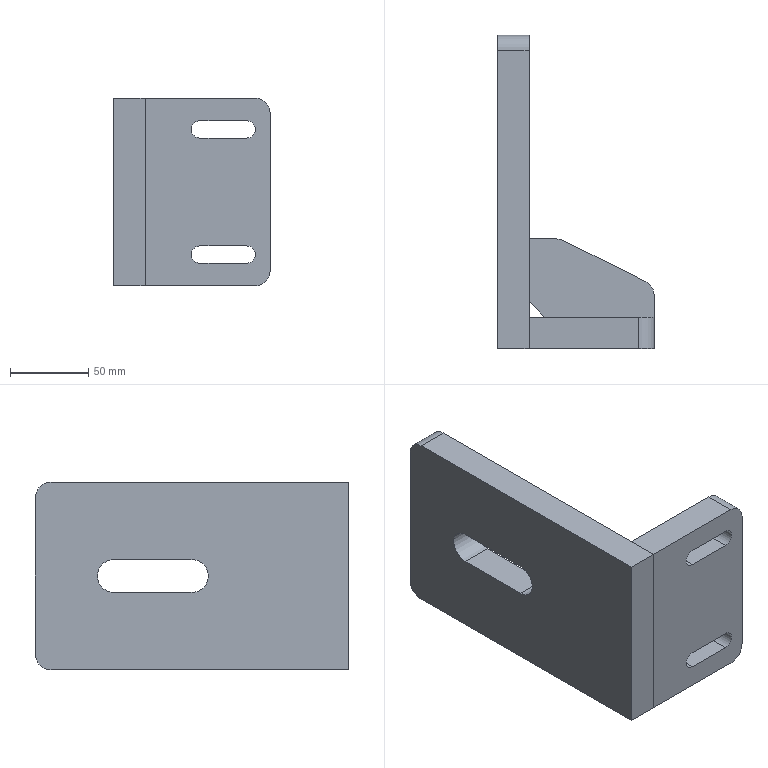Part | SolidWorks | features BaseBody 3 | 3 solids | 38 faces | box 100 x 200 x 120 mm | volume 655786 mm3 | plane 26 | cylinder 12 | commonest cylinder face diameters 20 x6 11 x4 21 x2
STEP:
#1=CARTESIAN_POINT('',(10.,-100.,-60.));
#2=VERTEX_POINT('',#1);
#3=CARTESIAN_POINT('',(10.,90.,-60.));
#4=VERTEX_POINT('',#3);
#5=CARTESIAN_POINT('',(10.,90.,-60.));
#6=DIRECTION('',(0.,1.,0.));
#7=VECTOR('',#6,1000.);
#8=LINE('',#5,#7);
#9=EDGE_CURVE('',#2,#4,#8,.T.);
#10=ORIENTED_EDGE('',*,*,#9,.T.);
#11=CARTESIAN_POINT('',(10.,100.,-50.));
#12=VERTEX_POINT('',#11);
#13=CARTESIAN_POINT('',(10.,90.,-50.));
#14=DIRECTION('',(1.,0.,0.));
#15=DIRECTION('',(0.,0.,1.));
#16=AXIS2_PLACEMENT_3D('',#13,#14,#15);
#17=CIRCLE('',#16,10.);
#18=EDGE_CURVE('',#4,#12,#17,.T.);
#19=ORIENTED_EDGE('',*,*,#18,.T.);
#20=CARTESIAN_POINT('',(10.,100.,50.));
#21=VERTEX_POINT('',#20);
#22=CARTESIAN_POINT('',(10.,100.,50.));
#23=DIRECTION('',(0.,0.,1.));
#24=VECTOR('',#23,1000.);
#25=LINE('',#22,#24);
#26=EDGE_CURVE('',#12,#21,#25,.T.);
#27=ORIENTED_EDGE('',*,*,#26,.T.);
#28=CARTESIAN_POINT('',(10.,90.,60.));
#29=VERTEX_POINT('',#28);
#30=CARTESIAN_POINT('',(10.,90.,50.));
#31=DIRECTION('',(1.,0.,0.));
#32=DIRECTION('',(0.,0.,-1.));
#33=AXIS2_PLACEMENT_3D('',#30,#31,#32);
#34=CIRCLE('',#33,10.);
#35=EDGE_CURVE('',#21,#29,#34,.T.);
#36=ORIENTED_EDGE('',*,*,#35,.T.);
#37=CARTESIAN_POINT('',(10.,-100.,60.));
#38=VERTEX_POINT('',#37);
#39=CARTESIAN_POINT('',(10.,90.,60.));
#40=DIRECTION('',(0.,-1.,0.));
#41=VECTOR('',#40,1000.);
#42=LINE('',#39,#41);
#43=EDGE_CURVE('',#29,#38,#42,.T.);
#44=ORIENTED_EDGE('',*,*,#43,.T.);
#45=CARTESIAN_POINT('',(10.,-100.,60.));
#46=DIRECTION('',(0.,0.,-1.));
#47=VECTOR('',#46,1000.);
#48=LINE('',#45,#47);
#49=EDGE_CURVE('',#38,#2,#48,.T.);
#50=ORIENTED_EDGE('',*,*,#49,.T.);
#51=EDGE_LOOP('',(#10,#19,#27,#36,#44,#50));
#52=FACE_OUTER_BOUND('',#51,.T.);
#53=CARTESIAN_POINT('',(10.,50.,10.5));
#54=VERTEX_POINT('',#53);
#55=CARTESIAN_POINT('',(10.,0.,10.5));
#56=VERTEX_POINT('',#55);
#57=CARTESIAN_POINT('',(10.,50.,10.5));
#58=DIRECTION('',(0.,-1.,0.));
#59=VECTOR('',#58,1000.);
#60=LINE('',#57,#59);
#61=EDGE_CURVE('',#54,#56,#60,.T.);
#62=ORIENTED_EDGE('',*,*,#61,.F.);
#63=CARTESIAN_POINT('',(10.,50.,-10.5));
#64=VERTEX_POINT('',#63);
#65=CARTESIAN_POINT('',(10.,50.,0.));
#66=DIRECTION('',(1.,0.,0.));
#67=DIRECTION('',(0.,0.,-1.));
#68=AXIS2_PLACEMENT_3D('',#65,#66,#67);
#69=CIRCLE('',#68,10.5);
#70=EDGE_CURVE('',#64,#54,#69,.T.);
#71=ORIENTED_EDGE('',*,*,#70,.F.);
#72=CARTESIAN_POINT('',(10.,0.,-10.5));
#73=VERTEX_POINT('',#72);
#74=CARTESIAN_POINT('',(10.,50.,-10.5));
#75=DIRECTION('',(0.,1.,0.));
#76=VECTOR('',#75,1000.);
#77=LINE('',#74,#76);
#78=EDGE_CURVE('',#73,#64,#77,.T.);
#79=ORIENTED_EDGE('',*,*,#78,.F.);
#80=CARTESIAN_POINT('',(10.,0.,0.));
#81=DIRECTION('',(1.,0.,0.));
#82=DIRECTION('',(0.,0.,-1.));
#83=AXIS2_PLACEMENT_3D('',#80,#81,#82);
#84=CIRCLE('',#83,10.5);
#85=EDGE_CURVE('',#56,#73,#84,.T.);
#86=ORIENTED_EDGE('',*,*,#85,.F.);
#87=EDGE_LOOP('',(#62,#71,#79,#86));
#88=FACE_BOUND('',#87,.T.);
#89=CARTESIAN_POINT('',(10.,90.,50.));
#90=DIRECTION('',(1.,0.,0.));
#91=DIRECTION('',(0.,0.,-1.));
#92=AXIS2_PLACEMENT_3D('',#89,#90,#91);
#93=PLANE('',#92);
#94=ADVANCED_FACE('',(#52,#88),#93,.T.);
#95=CARTESIAN_POINT('',(-10.,-100.,-60.));
#96=VERTEX_POINT('',#95);
#97=CARTESIAN_POINT('',(-10.,90.,-60.));
#98=VERTEX_POINT('',#97);
#99=CARTESIAN_POINT('',(-10.,90.,-60.));
#100=DIRECTION('',(0.,1.,0.));
#101=VECTOR('',#100,1000.);
#102=LINE('',#99,#101);
#103=EDGE_CURVE('',#96,#98,#102,.T.);
#104=ORIENTED_EDGE('',*,*,#103,.F.);
#105=CARTESIAN_POINT('',(-10.,-100.,60.));
#106=VERTEX_POINT('',#105);
#107=CARTESIAN_POINT('',(-10.,-100.,60.));
#108=DIRECTION('',(0.,0.,-1.));
#109=VECTOR('',#108,1000.);
#110=LINE('',#107,#109);
#111=EDGE_CURVE('',#106,#96,#110,.T.);
#112=ORIENTED_EDGE('',*,*,#111,.F.);
#113=CARTESIAN_POINT('',(-10.,90.,60.));
#114=VERTEX_POINT('',#113);
#115=CARTESIAN_POINT('',(-10.,90.,60.));
#116=DIRECTION('',(0.,-1.,0.));
#117=VECTOR('',#116,1000.);
#118=LINE('',#115,#117);
#119=EDGE_CURVE('',#114,#106,#118,.T.);
#120=ORIENTED_EDGE('',*,*,#119,.F.);
#121=CARTESIAN_POINT('',(-10.,100.,50.));
#122=VERTEX_POINT('',#121);
#123=CARTESIAN_POINT('',(-10.,90.,50.));
#124=DIRECTION('',(1.,0.,0.));
#125=DIRECTION('',(0.,0.,-1.));
#126=AXIS2_PLACEMENT_3D('',#123,#124,#125);
#127=CIRCLE('',#126,10.);
#128=EDGE_CURVE('',#122,#114,#127,.T.);
#129=ORIENTED_EDGE('',*,*,#128,.F.);
#130=CARTESIAN_POINT('',(-10.,100.,-50.));
#131=VERTEX_POINT('',#130);
#132=CARTESIAN_POINT('',(-10.,100.,50.));
#133=DIRECTION('',(0.,0.,1.));
#134=VECTOR('',#133,1000.);
#135=LINE('',#132,#134);
#136=EDGE_CURVE('',#131,#122,#135,.T.);
#137=ORIENTED_EDGE('',*,*,#136,.F.);
#138=CARTESIAN_POINT('',(-10.,90.,-50.));
#139=DIRECTION('',(1.,0.,0.));
#140=DIRECTION('',(0.,0.,1.));
#141=AXIS2_PLACEMENT_3D('',#138,#139,#140);
#142=CIRCLE('',#141,10.);
#143=EDGE_CURVE('',#98,#131,#142,.T.);
#144=ORIENTED_EDGE('',*,*,#143,.F.);
#145=EDGE_LOOP('',(#104,#112,#120,#129,#137,#144));
#146=FACE_OUTER_BOUND('',#145,.T.);
#147=CARTESIAN_POINT('',(-10.,50.,-10.5));
#148=VERTEX_POINT('',#147);
#149=CARTESIAN_POINT('',(-10.,50.,10.5));
#150=VERTEX_POINT('',#149);
#151=CARTESIAN_POINT('',(-10.,50.,0.));
#152=DIRECTION('',(1.,0.,0.));
#153=DIRECTION('',(0.,0.,-1.));
#154=AXIS2_PLACEMENT_3D('',#151,#152,#153);
#155=CIRCLE('',#154,10.5);
#156=EDGE_CURVE('',#148,#150,#155,.T.);
#157=ORIENTED_EDGE('',*,*,#156,.T.);
#158=CARTESIAN_POINT('',(-10.,0.,10.5));
#159=VERTEX_POINT('',#158);
#160=CARTESIAN_POINT('',(-10.,50.,10.5));
#161=DIRECTION('',(0.,-1.,0.));
#162=VECTOR('',#161,1000.);
#163=LINE('',#160,#162);
#164=EDGE_CURVE('',#150,#159,#163,.T.);
#165=ORIENTED_EDGE('',*,*,#164,.T.);
#166=CARTESIAN_POINT('',(-10.,0.,-10.5));
#167=VERTEX_POINT('',#166);
#168=CARTESIAN_POINT('',(-10.,0.,0.));
#169=DIRECTION('',(1.,0.,0.));
#170=DIRECTION('',(0.,0.,-1.));
#171=AXIS2_PLACEMENT_3D('',#168,#169,#170);
#172=CIRCLE('',#171,10.5);
#173=EDGE_CURVE('',#159,#167,#172,.T.);
#174=ORIENTED_EDGE('',*,*,#173,.T.);
#175=CARTESIAN_POINT('',(-10.,50.,-10.5));
#176=DIRECTION('',(0.,1.,0.));
#177=VECTOR('',#176,1000.);
#178=LINE('',#175,#177);
#179=EDGE_CURVE('',#167,#148,#178,.T.);
#180=ORIENTED_EDGE('',*,*,#179,.T.);
#181=EDGE_LOOP('',(#157,#165,#174,#180));
#182=FACE_BOUND('',#181,.T.);
#183=CARTESIAN_POINT('',(-10.,90.,50.));
#184=DIRECTION('',(1.,0.,0.));
#185=DIRECTION('',(0.,0.,-1.));
#186=AXIS2_PLACEMENT_3D('',#183,#184,#185);
#187=PLANE('',#186);
#188=ADVANCED_FACE('',(#146,#182),#187,.F.);
#189=ORIENTED_EDGE('',*,*,#103,.T.);
#190=CARTESIAN_POINT('',(10.,90.,-60.));
#191=DIRECTION('',(-1.,0.,0.));
#192=VECTOR('',#191,1000.);
#193=LINE('',#190,#192);
#194=EDGE_CURVE('',#4,#98,#193,.T.);
#195=ORIENTED_EDGE('',*,*,#194,.F.);
#196=ORIENTED_EDGE('',*,*,#9,.F.);
#197=CARTESIAN_POINT('',(10.,-100.,-60.));
#198=DIRECTION('',(-1.,0.,0.));
#199=VECTOR('',#198,1000.);
#200=LINE('',#197,#199);
#201=EDGE_CURVE('',#2,#96,#200,.T.);
#202=ORIENTED_EDGE('',*,*,#201,.T.);
#203=EDGE_LOOP('',(#189,#195,#196,#202));
#204=FACE_OUTER_BOUND('',#203,.T.);
#205=CARTESIAN_POINT('',(10.,90.,-60.));
#206=DIRECTION('',(0.,0.,1.));
#207=DIRECTION('',(0.,-1.,0.));
#208=AXIS2_PLACEMENT_3D('',#205,#206,#207);
#209=PLANE('',#208);
#210=ADVANCED_FACE('',(#204),#209,.F.);
#211=ORIENTED_EDGE('',*,*,#143,.T.);
#212=CARTESIAN_POINT('',(10.,100.,-50.));
#213=DIRECTION('',(-1.,0.,0.));
#214=VECTOR('',#213,1000.);
#215=LINE('',#212,#214);
#216=EDGE_CURVE('',#12,#131,#215,.T.);
#217=ORIENTED_EDGE('',*,*,#216,.F.);
#218=ORIENTED_EDGE('',*,*,#18,.F.);
#219=ORIENTED_EDGE('',*,*,#194,.T.);
#220=EDGE_LOOP('',(#211,#217,#218,#219));
#221=FACE_OUTER_BOUND('',#220,.T.);
#222=CARTESIAN_POINT('',(10.,90.,-50.));
#223=DIRECTION('',(-1.,0.,0.));
#224=DIRECTION('',(0.,0.,1.));
#225=AXIS2_PLACEMENT_3D('',#222,#223,#224);
#226=CYLINDRICAL_SURFACE('',#225,10.);
#227=ADVANCED_FACE('',(#221),#226,.T.);
#228=ORIENTED_EDGE('',*,*,#136,.T.);
#229=CARTESIAN_POINT('',(10.,100.,50.));
#230=DIRECTION('',(-1.,0.,0.));
#231=VECTOR('',#230,1000.);
#232=LINE('',#229,#231);
#233=EDGE_CURVE('',#21,#122,#232,.T.);
#234=ORIENTED_EDGE('',*,*,#233,.F.);
#235=ORIENTED_EDGE('',*,*,#26,.F.);
#236=ORIENTED_EDGE('',*,*,#216,.T.);
#237=EDGE_LOOP('',(#228,#234,#235,#236));
#238=FACE_OUTER_BOUND('',#237,.T.);
#239=CARTESIAN_POINT('',(10.,100.,50.));
#240=DIRECTION('',(0.,-1.,0.));
#241=DIRECTION('',(0.,0.,-1.));
#242=AXIS2_PLACEMENT_3D('',#239,#240,#241);
#243=PLANE('',#242);
#244=ADVANCED_FACE('',(#238),#243,.F.);
#245=ORIENTED_EDGE('',*,*,#128,.T.);
#246=CARTESIAN_POINT('',(10.,90.,60.));
#247=DIRECTION('',(-1.,0.,0.));
#248=VECTOR('',#247,1000.);
#249=LINE('',#246,#248);
#250=EDGE_CURVE('',#29,#114,#249,.T.);
#251=ORIENTED_EDGE('',*,*,#250,.F.);
#252=ORIENTED_EDGE('',*,*,#35,.F.);
#253=ORIENTED_EDGE('',*,*,#233,.T.);
#254=EDGE_LOOP('',(#245,#251,#252,#253));
#255=FACE_OUTER_BOUND('',#254,.T.);
#256=CARTESIAN_POINT('',(10.,90.,50.));
#257=DIRECTION('',(-1.,0.,0.));
#258=DIRECTION('',(0.,0.,1.));
#259=AXIS2_PLACEMENT_3D('',#256,#257,#258);
#260=CYLINDRICAL_SURFACE('',#259,10.);
#261=ADVANCED_FACE('',(#255),#260,.T.);
#262=ORIENTED_EDGE('',*,*,#119,.T.);
#263=CARTESIAN_POINT('',(10.,-100.,60.));
#264=DIRECTION('',(-1.,0.,0.));
#265=VECTOR('',#264,1000.);
#266=LINE('',#263,#265);
#267=EDGE_CURVE('',#38,#106,#266,.T.);
#268=ORIENTED_EDGE('',*,*,#267,.F.);
#269=ORIENTED_EDGE('',*,*,#43,.F.);
#270=ORIENTED_EDGE('',*,*,#250,.T.);
#271=EDGE_LOOP('',(#262,#268,#269,#270));
#272=FACE_OUTER_BOUND('',#271,.T.);
#273=CARTESIAN_POINT('',(10.,90.,60.));
#274=DIRECTION('',(0.,0.,-1.));
#275=DIRECTION('',(0.,1.,0.));
#276=AXIS2_PLACEMENT_3D('',#273,#274,#275);
#277=PLANE('',#276);
#278=ADVANCED_FACE('',(#272),#277,.F.);
#279=ORIENTED_EDGE('',*,*,#111,.T.);
#280=ORIENTED_EDGE('',*,*,#201,.F.);
#281=ORIENTED_EDGE('',*,*,#49,.F.);
#282=ORIENTED_EDGE('',*,*,#267,.T.);
#283=EDGE_LOOP('',(#279,#280,#281,#282));
#284=FACE_OUTER_BOUND('',#283,.T.);
#285=CARTESIAN_POINT('',(10.,-100.,60.));
#286=DIRECTION('',(0.,1.,0.));
#287=DIRECTION('',(0.,0.,1.));
#288=AXIS2_PLACEMENT_3D('',#285,#286,#287);
#289=PLANE('',#288);
#290=ADVANCED_FACE('',(#284),#289,.F.);
#291=ORIENTED_EDGE('',*,*,#156,.F.);
#292=CARTESIAN_POINT('',(10.,50.,-10.5));
#293=DIRECTION('',(-1.,0.,0.));
#294=VECTOR('',#293,1000.);
#295=LINE('',#292,#294);
#296=EDGE_CURVE('',#64,#148,#295,.T.);
#297=ORIENTED_EDGE('',*,*,#296,.F.);
#298=ORIENTED_EDGE('',*,*,#70,.T.);
#299=CARTESIAN_POINT('',(10.,50.,10.5));
#300=DIRECTION('',(-1.,0.,0.));
#301=VECTOR('',#300,1000.);
#302=LINE('',#299,#301);
#303=EDGE_CURVE('',#54,#150,#302,.T.);
#304=ORIENTED_EDGE('',*,*,#303,.T.);
#305=EDGE_LOOP('',(#291,#297,#298,#304));
#306=FACE_OUTER_BOUND('',#305,.T.);
#307=CARTESIAN_POINT('',(10.,50.,0.));
#308=DIRECTION('',(-1.,0.,0.));
#309=DIRECTION('',(0.,0.,1.));
#310=AXIS2_PLACEMENT_3D('',#307,#308,#309);
#311=CYLINDRICAL_SURFACE('',#310,10.5);
#312=ADVANCED_FACE('',(#306),#311,.F.);
#313=ORIENTED_EDGE('',*,*,#164,.F.);
#314=ORIENTED_EDGE('',*,*,#303,.F.);
#315=ORIENTED_EDGE('',*,*,#61,.T.);
#316=CARTESIAN_POINT('',(10.,0.,10.5));
#317=DIRECTION('',(-1.,0.,0.));
#318=VECTOR('',#317,1000.);
#319=LINE('',#316,#318);
#320=EDGE_CURVE('',#56,#159,#319,.T.);
#321=ORIENTED_EDGE('',*,*,#320,.T.);
#322=EDGE_LOOP('',(#313,#314,#315,#321));
#323=FACE_OUTER_BOUND('',#322,.T.);
#324=CARTESIAN_POINT('',(10.,50.,10.5));
#325=DIRECTION('',(0.,0.,-1.));
#326=DIRECTION('',(0.,1.,0.));
#327=AXIS2_PLACEMENT_3D('',#324,#325,#326);
#328=PLANE('',#327);
#329=ADVANCED_FACE('',(#323),#328,.T.);
#330=ORIENTED_EDGE('',*,*,#173,.F.);
#331=ORIENTED_EDGE('',*,*,#320,.F.);
#332=ORIENTED_EDGE('',*,*,#85,.T.);
#333=CARTESIAN_POINT('',(10.,0.,-10.5));
#334=DIRECTION('',(-1.,0.,0.));
#335=VECTOR('',#334,1000.);
#336=LINE('',#333,#335);
#337=EDGE_CURVE('',#73,#167,#336,.T.);
#338=ORIENTED_EDGE('',*,*,#337,.T.);
#339=EDGE_LOOP('',(#330,#331,#332,#338));
#340=FACE_OUTER_BOUND('',#339,.T.);
#341=CARTESIAN_POINT('',(10.,0.,0.));
#342=DIRECTION('',(-1.,0.,0.));
#343=DIRECTION('',(0.,0.,1.));
#344=AXIS2_PLACEMENT_3D('',#341,#342,#343);
#345=CYLINDRICAL_SURFACE('',#344,10.5);
#346=ADVANCED_FACE('',(#340),#345,.F.);
#347=ORIENTED_EDGE('',*,*,#179,.F.);
#348=ORIENTED_EDGE('',*,*,#337,.F.);
#349=ORIENTED_EDGE('',*,*,#78,.T.);
#350=ORIENTED_EDGE('',*,*,#296,.T.);
#351=EDGE_LOOP('',(#347,#348,#349,#350));
#352=FACE_OUTER_BOUND('',#351,.T.);
#353=CARTESIAN_POINT('',(10.,50.,-10.5));
#354=DIRECTION('',(0.,0.,1.));
#355=DIRECTION('',(0.,-1.,0.));
#356=AXIS2_PLACEMENT_3D('',#353,#354,#355);
#357=PLANE('',#356);
#358=ADVANCED_FACE('',(#352),#357,.T.);
#359=CLOSED_SHELL('',(#94,#188,#210,#227,#244,#261,#278,#290,#312,#329,#346,#358));
#360=MANIFOLD_SOLID_BREP('',#359);
#361=CARTESIAN_POINT('',(80.,-100.,60.));
#362=VERTEX_POINT('',#361);
#363=CARTESIAN_POINT('',(10.,-100.,60.));
#364=VERTEX_POINT('',#363);
#365=CARTESIAN_POINT('',(90.,-100.,60.));
#366=DIRECTION('',(-1.,0.,0.));
#367=VECTOR('',#366,1000.);
#368=LINE('',#365,#367);
#369=EDGE_CURVE('',#362,#364,#368,.T.);
#370=ORIENTED_EDGE('',*,*,#369,.F.);
#371=CARTESIAN_POINT('',(80.,-80.,60.));
#372=VERTEX_POINT('',#371);
#373=CARTESIAN_POINT('',(80.,-100.,60.));
#374=DIRECTION('',(0.,1.,0.));
#375=VECTOR('',#374,1000.);
#376=LINE('',#373,#375);
#377=EDGE_CURVE('',#362,#372,#376,.T.);
#378=ORIENTED_EDGE('',*,*,#377,.T.);
#379=CARTESIAN_POINT('',(10.,-80.,60.));
#380=VERTEX_POINT('',#379);
#381=CARTESIAN_POINT('',(90.,-80.,60.));
#382=DIRECTION('',(-1.,0.,0.));
#383=VECTOR('',#382,1000.);
#384=LINE('',#381,#383);
#385=EDGE_CURVE('',#372,#380,#384,.T.);
#386=ORIENTED_EDGE('',*,*,#385,.T.);
#387=CARTESIAN_POINT('',(10.,-100.,60.));
#388=DIRECTION('',(0.,-1.,0.));
#389=VECTOR('',#388,1000.);
#390=LINE('',#387,#389);
#391=EDGE_CURVE('',#380,#364,#390,.T.);
#392=ORIENTED_EDGE('',*,*,#391,.T.);
#393=EDGE_LOOP('',(#370,#378,#386,#392));
#394=FACE_OUTER_BOUND('',#393,.T.);
#395=CARTESIAN_POINT('',(90.,-100.,60.));
#396=DIRECTION('',(0.,0.,-1.));
#397=DIRECTION('',(-1.,0.,0.));
#398=AXIS2_PLACEMENT_3D('',#395,#396,#397);
#399=PLANE('',#398);
#400=ADVANCED_FACE('',(#394),#399,.F.);
#401=CARTESIAN_POINT('',(75.,-100.,-45.5));
#402=VERTEX_POINT('',#401);
#403=CARTESIAN_POINT('',(45.,-100.,-45.5));
#404=VERTEX_POINT('',#403);
#405=CARTESIAN_POINT('',(90.,-100.,-45.5));
#406=DIRECTION('',(-1.,0.,0.));
#407=VECTOR('',#406,1000.);
#408=LINE('',#405,#407);
#409=EDGE_CURVE('',#402,#404,#408,.T.);
#410=ORIENTED_EDGE('',*,*,#409,.T.);
#411=CARTESIAN_POINT('',(45.,-100.,-34.5));
#412=VERTEX_POINT('',#411);
#413=CARTESIAN_POINT('',(45.,-100.,-40.));
#414=DIRECTION('',(0.,1.,0.));
#415=DIRECTION('',(0.,0.,1.));
#416=AXIS2_PLACEMENT_3D('',#413,#414,#415);
#417=CIRCLE('',#416,5.5);
#418=EDGE_CURVE('',#404,#412,#417,.T.);
#419=ORIENTED_EDGE('',*,*,#418,.T.);
#420=CARTESIAN_POINT('',(75.,-100.,-34.5));
#421=VERTEX_POINT('',#420);
#422=CARTESIAN_POINT('',(90.,-100.,-34.5));
#423=DIRECTION('',(1.,0.,0.));
#424=VECTOR('',#423,1000.);
#425=LINE('',#422,#424);
#426=EDGE_CURVE('',#412,#421,#425,.T.);
#427=ORIENTED_EDGE('',*,*,#426,.T.);
#428=CARTESIAN_POINT('',(75.,-100.,-40.));
#429=DIRECTION('',(0.,1.,0.));
#430=DIRECTION('',(0.,0.,1.));
#431=AXIS2_PLACEMENT_3D('',#428,#429,#430);
#432=CIRCLE('',#431,5.5);
#433=EDGE_CURVE('',#421,#402,#432,.T.);
#434=ORIENTED_EDGE('',*,*,#433,.T.);
#435=EDGE_LOOP('',(#410,#419,#427,#434));
#436=FACE_BOUND('',#435,.T.);
#437=CARTESIAN_POINT('',(75.,-100.,34.5));
#438=VERTEX_POINT('',#437);
#439=CARTESIAN_POINT('',(45.,-100.,34.5));
#440=VERTEX_POINT('',#439);
#441=CARTESIAN_POINT('',(90.,-100.,34.5));
#442=DIRECTION('',(-1.,0.,0.));
#443=VECTOR('',#442,1000.);
#444=LINE('',#441,#443);
#445=EDGE_CURVE('',#438,#440,#444,.T.);
#446=ORIENTED_EDGE('',*,*,#445,.T.);
#447=CARTESIAN_POINT('',(45.,-100.,45.5));
#448=VERTEX_POINT('',#447);
#449=CARTESIAN_POINT('',(45.,-100.,40.));
#450=DIRECTION('',(0.,1.,0.));
#451=DIRECTION('',(0.,0.,1.));
#452=AXIS2_PLACEMENT_3D('',#449,#450,#451);
#453=CIRCLE('',#452,5.5);
#454=EDGE_CURVE('',#440,#448,#453,.T.);
#455=ORIENTED_EDGE('',*,*,#454,.T.);
#456=CARTESIAN_POINT('',(75.,-100.,45.5));
#457=VERTEX_POINT('',#456);
#458=CARTESIAN_POINT('',(90.,-100.,45.5));
#459=DIRECTION('',(1.,0.,0.));
#460=VECTOR('',#459,1000.);
#461=LINE('',#458,#460);
#462=EDGE_CURVE('',#448,#457,#461,.T.);
#463=ORIENTED_EDGE('',*,*,#462,.T.);
#464=CARTESIAN_POINT('',(75.,-100.,40.));
#465=DIRECTION('',(0.,1.,0.));
#466=DIRECTION('',(0.,0.,1.));
#467=AXIS2_PLACEMENT_3D('',#464,#465,#466);
#468=CIRCLE('',#467,5.5);
#469=EDGE_CURVE('',#457,#438,#468,.T.);
#470=ORIENTED_EDGE('',*,*,#469,.T.);
#471=EDGE_LOOP('',(#446,#455,#463,#470));
#472=FACE_BOUND('',#471,.T.);
#473=CARTESIAN_POINT('',(90.,-100.,50.));
#474=VERTEX_POINT('',#473);
#475=CARTESIAN_POINT('',(90.,-100.,-50.));
#476=VERTEX_POINT('',#475);
#477=CARTESIAN_POINT('',(90.,-100.,60.));
#478=DIRECTION('',(0.,0.,-1.));
#479=VECTOR('',#478,1000.);
#480=LINE('',#477,#479);
#481=EDGE_CURVE('',#474,#476,#480,.T.);
#482=ORIENTED_EDGE('',*,*,#481,.F.);
#483=CARTESIAN_POINT('',(80.,-100.,50.));
#484=DIRECTION('',(0.,-1.,0.));
#485=DIRECTION('',(0.,0.,1.));
#486=AXIS2_PLACEMENT_3D('',#483,#484,#485);
#487=CIRCLE('',#486,10.);
#488=EDGE_CURVE('',#474,#362,#487,.T.);
#489=ORIENTED_EDGE('',*,*,#488,.T.);
#490=ORIENTED_EDGE('',*,*,#369,.T.);
#491=CARTESIAN_POINT('',(10.,-100.,-60.));
#492=VERTEX_POINT('',#491);
#493=CARTESIAN_POINT('',(10.,-100.,60.));
#494=DIRECTION('',(0.,0.,-1.));
#495=VECTOR('',#494,1000.);
#496=LINE('',#493,#495);
#497=EDGE_CURVE('',#364,#492,#496,.T.);
#498=ORIENTED_EDGE('',*,*,#497,.T.);
#499=CARTESIAN_POINT('',(80.,-100.,-60.));
#500=VERTEX_POINT('',#499);
#501=CARTESIAN_POINT('',(90.,-100.,-60.));
#502=DIRECTION('',(-1.,0.,0.));
#503=VECTOR('',#502,1000.);
#504=LINE('',#501,#503);
#505=EDGE_CURVE('',#500,#492,#504,.T.);
#506=ORIENTED_EDGE('',*,*,#505,.F.);
#507=CARTESIAN_POINT('',(80.,-100.,-50.));
#508=DIRECTION('',(0.,-1.,0.));
#509=DIRECTION('',(0.,0.,1.));
#510=AXIS2_PLACEMENT_3D('',#507,#508,#509);
#511=CIRCLE('',#510,10.);
#512=EDGE_CURVE('',#500,#476,#511,.T.);
#513=ORIENTED_EDGE('',*,*,#512,.T.);
#514=EDGE_LOOP('',(#482,#489,#490,#498,#506,#513));
#515=FACE_OUTER_BOUND('',#514,.T.);
#516=CARTESIAN_POINT('',(90.,-100.,60.));
#517=DIRECTION('',(0.,1.,0.));
#518=DIRECTION('',(0.,0.,1.));
#519=AXIS2_PLACEMENT_3D('',#516,#517,#518);
#520=PLANE('',#519);
#521=ADVANCED_FACE('',(#436,#472,#515),#520,.F.);
#522=CARTESIAN_POINT('',(80.,-80.,-60.));
#523=VERTEX_POINT('',#522);
#524=CARTESIAN_POINT('',(10.,-80.,-60.));
#525=VERTEX_POINT('',#524);
#526=CARTESIAN_POINT('',(90.,-80.,-60.));
#527=DIRECTION('',(-1.,0.,0.));
#528=VECTOR('',#527,1000.);
#529=LINE('',#526,#528);
#530=EDGE_CURVE('',#523,#525,#529,.T.);
#531=ORIENTED_EDGE('',*,*,#530,.F.);
#532=CARTESIAN_POINT('',(80.,-100.,-60.));
#533=DIRECTION('',(0.,-1.,0.));
#534=VECTOR('',#533,1000.);
#535=LINE('',#532,#534);
#536=EDGE_CURVE('',#523,#500,#535,.T.);
#537=ORIENTED_EDGE('',*,*,#536,.T.);
#538=ORIENTED_EDGE('',*,*,#505,.T.);
#539=CARTESIAN_POINT('',(10.,-100.,-60.));
#540=DIRECTION('',(0.,1.,0.));
#541=VECTOR('',#540,1000.);
#542=LINE('',#539,#541);
#543=EDGE_CURVE('',#492,#525,#542,.T.);
#544=ORIENTED_EDGE('',*,*,#543,.T.);
#545=EDGE_LOOP('',(#531,#537,#538,#544));
#546=FACE_OUTER_BOUND('',#545,.T.);
#547=CARTESIAN_POINT('',(90.,-100.,-60.));
#548=DIRECTION('',(0.,0.,1.));
#549=DIRECTION('',(0.,-1.,0.));
#550=AXIS2_PLACEMENT_3D('',#547,#548,#549);
#551=PLANE('',#550);
#552=ADVANCED_FACE('',(#546),#551,.F.);
#553=CARTESIAN_POINT('',(45.,-80.,-34.5));
#554=VERTEX_POINT('',#553);
#555=CARTESIAN_POINT('',(75.,-80.,-34.5));
#556=VERTEX_POINT('',#555);
#557=CARTESIAN_POINT('',(45.,-80.,-34.5));
#558=DIRECTION('',(1.,0.,0.));
#559=VECTOR('',#558,1000.);
#560=LINE('',#557,#559);
#561=EDGE_CURVE('',#554,#556,#560,.T.);
#562=ORIENTED_EDGE('',*,*,#561,.F.);
#563=CARTESIAN_POINT('',(45.,-80.,-45.5));
#564=VERTEX_POINT('',#563);
#565=CARTESIAN_POINT('',(45.,-80.,-40.));
#566=DIRECTION('',(0.,1.,0.));
#567=DIRECTION('',(0.,0.,1.));
#568=AXIS2_PLACEMENT_3D('',#565,#566,#567);
#569=CIRCLE('',#568,5.5);
#570=EDGE_CURVE('',#564,#554,#569,.T.);
#571=ORIENTED_EDGE('',*,*,#570,.F.);
#572=CARTESIAN_POINT('',(75.,-80.,-45.5));
#573=VERTEX_POINT('',#572);
#574=CARTESIAN_POINT('',(45.,-80.,-45.5));
#575=DIRECTION('',(-1.,0.,0.));
#576=VECTOR('',#575,1000.);
#577=LINE('',#574,#576);
#578=EDGE_CURVE('',#573,#564,#577,.T.);
#579=ORIENTED_EDGE('',*,*,#578,.F.);
#580=CARTESIAN_POINT('',(75.,-80.,-40.));
#581=DIRECTION('',(0.,1.,0.));
#582=DIRECTION('',(0.,0.,1.));
#583=AXIS2_PLACEMENT_3D('',#580,#581,#582);
#584=CIRCLE('',#583,5.5);
#585=EDGE_CURVE('',#556,#573,#584,.T.);
#586=ORIENTED_EDGE('',*,*,#585,.F.);
#587=EDGE_LOOP('',(#562,#571,#579,#586));
#588=FACE_BOUND('',#587,.T.);
#589=CARTESIAN_POINT('',(45.,-80.,45.5));
#590=VERTEX_POINT('',#589);
#591=CARTESIAN_POINT('',(75.,-80.,45.5));
#592=VERTEX_POINT('',#591);
#593=CARTESIAN_POINT('',(45.,-80.,45.5));
#594=DIRECTION('',(1.,0.,0.));
#595=VECTOR('',#594,1000.);
#596=LINE('',#593,#595);
#597=EDGE_CURVE('',#590,#592,#596,.T.);
#598=ORIENTED_EDGE('',*,*,#597,.F.);
#599=CARTESIAN_POINT('',(45.,-80.,34.5));
#600=VERTEX_POINT('',#599);
#601=CARTESIAN_POINT('',(45.,-80.,40.));
#602=DIRECTION('',(0.,1.,0.));
#603=DIRECTION('',(0.,0.,1.));
#604=AXIS2_PLACEMENT_3D('',#601,#602,#603);
#605=CIRCLE('',#604,5.5);
#606=EDGE_CURVE('',#600,#590,#605,.T.);
#607=ORIENTED_EDGE('',*,*,#606,.F.);
#608=CARTESIAN_POINT('',(75.,-80.,34.5));
#609=VERTEX_POINT('',#608);
#610=CARTESIAN_POINT('',(45.,-80.,34.5));
#611=DIRECTION('',(-1.,0.,0.));
#612=VECTOR('',#611,1000.);
#613=LINE('',#610,#612);
#614=EDGE_CURVE('',#609,#600,#613,.T.);
#615=ORIENTED_EDGE('',*,*,#614,.F.);
#616=CARTESIAN_POINT('',(75.,-80.,40.));
#617=DIRECTION('',(0.,1.,0.));
#618=DIRECTION('',(0.,0.,1.));
#619=AXIS2_PLACEMENT_3D('',#616,#617,#618);
#620=CIRCLE('',#619,5.5);
#621=EDGE_CURVE('',#592,#609,#620,.T.);
#622=ORIENTED_EDGE('',*,*,#621,.F.);
#623=EDGE_LOOP('',(#598,#607,#615,#622));
#624=FACE_BOUND('',#623,.T.);
#625=ORIENTED_EDGE('',*,*,#385,.F.);
#626=CARTESIAN_POINT('',(90.,-80.,50.));
#627=VERTEX_POINT('',#626);
#628=CARTESIAN_POINT('',(80.,-80.,50.));
#629=DIRECTION('',(0.,1.,0.));
#630=DIRECTION('',(0.,0.,-1.));
#631=AXIS2_PLACEMENT_3D('',#628,#629,#630);
#632=CIRCLE('',#631,10.);
#633=EDGE_CURVE('',#372,#627,#632,.T.);
#634=ORIENTED_EDGE('',*,*,#633,.T.);
#635=CARTESIAN_POINT('',(90.,-80.,-50.));
#636=VERTEX_POINT('',#635);
#637=CARTESIAN_POINT('',(90.,-80.,60.));
#638=DIRECTION('',(0.,0.,1.));
#639=VECTOR('',#638,1000.);
#640=LINE('',#637,#639);
#641=EDGE_CURVE('',#636,#627,#640,.T.);
#642=ORIENTED_EDGE('',*,*,#641,.F.);
#643=CARTESIAN_POINT('',(80.,-80.,-50.));
#644=DIRECTION('',(0.,1.,0.));
#645=DIRECTION('',(0.,0.,-1.));
#646=AXIS2_PLACEMENT_3D('',#643,#644,#645);
#647=CIRCLE('',#646,10.);
#648=EDGE_CURVE('',#636,#523,#647,.T.);
#649=ORIENTED_EDGE('',*,*,#648,.T.);
#650=ORIENTED_EDGE('',*,*,#530,.T.);
#651=CARTESIAN_POINT('',(10.,-80.,60.));
#652=DIRECTION('',(0.,0.,1.));
#653=VECTOR('',#652,1000.);
#654=LINE('',#651,#653);
#655=EDGE_CURVE('',#525,#380,#654,.T.);
#656=ORIENTED_EDGE('',*,*,#655,.T.);
#657=EDGE_LOOP('',(#625,#634,#642,#649,#650,#656));
#658=FACE_OUTER_BOUND('',#657,.T.);
#659=CARTESIAN_POINT('',(90.,-80.,60.));
#660=DIRECTION('',(0.,-1.,0.));
#661=DIRECTION('',(0.,0.,-1.));
#662=AXIS2_PLACEMENT_3D('',#659,#660,#661);
#663=PLANE('',#662);
#664=ADVANCED_FACE('',(#588,#624,#658),#663,.F.);
#665=ORIENTED_EDGE('',*,*,#641,.T.);
#666=CARTESIAN_POINT('',(90.,0.,50.));
#667=DIRECTION('',(0.,-1.,0.));
#668=VECTOR('',#667,1000.);
#669=LINE('',#666,#668);
#670=EDGE_CURVE('',#627,#474,#669,.T.);
#671=ORIENTED_EDGE('',*,*,#670,.T.);
#672=ORIENTED_EDGE('',*,*,#481,.T.);
#673=CARTESIAN_POINT('',(90.,0.,-50.));
#674=DIRECTION('',(0.,1.,0.));
#675=VECTOR('',#674,1000.);
#676=LINE('',#673,#675);
#677=EDGE_CURVE('',#476,#636,#676,.T.);
#678=ORIENTED_EDGE('',*,*,#677,.T.);
#679=EDGE_LOOP('',(#665,#671,#672,#678));
#680=FACE_OUTER_BOUND('',#679,.T.);
#681=CARTESIAN_POINT('',(90.,0.,0.));
#682=DIRECTION('',(-1.,0.,0.));
#683=DIRECTION('',(0.,0.,1.));
#684=AXIS2_PLACEMENT_3D('',#681,#682,#683);
#685=PLANE('',#684);
#686=ADVANCED_FACE('',(#680),#685,.F.);
#687=ORIENTED_EDGE('',*,*,#391,.F.);
#688=ORIENTED_EDGE('',*,*,#655,.F.);
#689=ORIENTED_EDGE('',*,*,#543,.F.);
#690=ORIENTED_EDGE('',*,*,#497,.F.);
#691=EDGE_LOOP('',(#687,#688,#689,#690));
#692=FACE_OUTER_BOUND('',#691,.T.);
#693=CARTESIAN_POINT('',(10.,0.,0.));
#694=DIRECTION('',(-1.,0.,0.));
#695=DIRECTION('',(0.,0.,1.));
#696=AXIS2_PLACEMENT_3D('',#693,#694,#695);
#697=PLANE('',#696);
#698=ADVANCED_FACE('',(#692),#697,.T.);
#699=ORIENTED_EDGE('',*,*,#633,.F.);
#700=ORIENTED_EDGE('',*,*,#377,.F.);
#701=ORIENTED_EDGE('',*,*,#488,.F.);
#702=ORIENTED_EDGE('',*,*,#670,.F.);
#703=EDGE_LOOP('',(#699,#700,#701,#702));
#704=FACE_OUTER_BOUND('',#703,.T.);
#705=CARTESIAN_POINT('',(80.,0.,50.));
#706=DIRECTION('',(0.,-1.,0.));
#707=DIRECTION('',(0.,0.,-1.));
#708=AXIS2_PLACEMENT_3D('',#705,#706,#707);
#709=CYLINDRICAL_SURFACE('',#708,10.);
#710=ADVANCED_FACE('',(#704),#709,.T.);
#711=ORIENTED_EDGE('',*,*,#512,.F.);
#712=ORIENTED_EDGE('',*,*,#536,.F.);
#713=ORIENTED_EDGE('',*,*,#648,.F.);
#714=ORIENTED_EDGE('',*,*,#677,.F.);
#715=EDGE_LOOP('',(#711,#712,#713,#714));
#716=FACE_OUTER_BOUND('',#715,.T.);
#717=CARTESIAN_POINT('',(80.,0.,-50.));
#718=DIRECTION('',(0.,1.,0.));
#719=DIRECTION('',(0.,0.,1.));
#720=AXIS2_PLACEMENT_3D('',#717,#718,#719);
#721=CYLINDRICAL_SURFACE('',#720,10.);
#722=ADVANCED_FACE('',(#716),#721,.T.);
#723=CARTESIAN_POINT('',(45.,-140.,34.5));
#724=DIRECTION('',(0.,1.,0.));
#725=VECTOR('',#724,1000.);
#726=LINE('',#723,#725);
#727=EDGE_CURVE('',#440,#600,#726,.T.);
#728=ORIENTED_EDGE('',*,*,#727,.T.);
#729=ORIENTED_EDGE('',*,*,#606,.T.);
#730=CARTESIAN_POINT('',(45.,-140.,45.5));
#731=DIRECTION('',(0.,1.,0.));
#732=VECTOR('',#731,1000.);
#733=LINE('',#730,#732);
#734=EDGE_CURVE('',#448,#590,#733,.T.);
#735=ORIENTED_EDGE('',*,*,#734,.F.);
#736=ORIENTED_EDGE('',*,*,#454,.F.);
#737=EDGE_LOOP('',(#728,#729,#735,#736));
#738=FACE_OUTER_BOUND('',#737,.T.);
#739=CARTESIAN_POINT('',(45.,-140.,40.));
#740=DIRECTION('',(0.,1.,0.));
#741=DIRECTION('',(0.,0.,1.));
#742=AXIS2_PLACEMENT_3D('',#739,#740,#741);
#743=CYLINDRICAL_SURFACE('',#742,5.5);
#744=ADVANCED_FACE('',(#738),#743,.F.);
#745=CARTESIAN_POINT('',(75.,-140.,34.5));
#746=DIRECTION('',(0.,1.,0.));
#747=VECTOR('',#746,1000.);
#748=LINE('',#745,#747);
#749=EDGE_CURVE('',#438,#609,#748,.T.);
#750=ORIENTED_EDGE('',*,*,#749,.T.);
#751=ORIENTED_EDGE('',*,*,#614,.T.);
#752=ORIENTED_EDGE('',*,*,#727,.F.);
#753=ORIENTED_EDGE('',*,*,#445,.F.);
#754=EDGE_LOOP('',(#750,#751,#752,#753));
#755=FACE_OUTER_BOUND('',#754,.T.);
#756=CARTESIAN_POINT('',(45.,-140.,34.5));
#757=DIRECTION('',(0.,0.,-1.));
#758=DIRECTION('',(-1.,0.,0.));
#759=AXIS2_PLACEMENT_3D('',#756,#757,#758);
#760=PLANE('',#759);
#761=ADVANCED_FACE('',(#755),#760,.F.);
#762=CARTESIAN_POINT('',(75.,-140.,45.5));
#763=DIRECTION('',(0.,1.,0.));
#764=VECTOR('',#763,1000.);
#765=LINE('',#762,#764);
#766=EDGE_CURVE('',#457,#592,#765,.T.);
#767=ORIENTED_EDGE('',*,*,#766,.T.);
#768=ORIENTED_EDGE('',*,*,#621,.T.);
#769=ORIENTED_EDGE('',*,*,#749,.F.);
#770=ORIENTED_EDGE('',*,*,#469,.F.);
#771=EDGE_LOOP('',(#767,#768,#769,#770));
#772=FACE_OUTER_BOUND('',#771,.T.);
#773=CARTESIAN_POINT('',(75.,-140.,40.));
#774=DIRECTION('',(0.,1.,0.));
#775=DIRECTION('',(0.,0.,1.));
#776=AXIS2_PLACEMENT_3D('',#773,#774,#775);
#777=CYLINDRICAL_SURFACE('',#776,5.5);
#778=ADVANCED_FACE('',(#772),#777,.F.);
#779=ORIENTED_EDGE('',*,*,#734,.T.);
#780=ORIENTED_EDGE('',*,*,#597,.T.);
#781=ORIENTED_EDGE('',*,*,#766,.F.);
#782=ORIENTED_EDGE('',*,*,#462,.F.);
#783=EDGE_LOOP('',(#779,#780,#781,#782));
#784=FACE_OUTER_BOUND('',#783,.T.);
#785=CARTESIAN_POINT('',(45.,-140.,45.5));
#786=DIRECTION('',(0.,0.,1.));
#787=DIRECTION('',(1.,0.,0.));
#788=AXIS2_PLACEMENT_3D('',#785,#786,#787);
#789=PLANE('',#788);
#790=ADVANCED_FACE('',(#784),#789,.F.);
#791=CARTESIAN_POINT('',(45.,-140.,-45.5));
#792=DIRECTION('',(0.,1.,0.));
#793=VECTOR('',#792,1000.);
#794=LINE('',#791,#793);
#795=EDGE_CURVE('',#404,#564,#794,.T.);
#796=ORIENTED_EDGE('',*,*,#795,.T.);
#797=ORIENTED_EDGE('',*,*,#570,.T.);
#798=CARTESIAN_POINT('',(45.,-140.,-34.5));
#799=DIRECTION('',(0.,1.,0.));
#800=VECTOR('',#799,1000.);
#801=LINE('',#798,#800);
#802=EDGE_CURVE('',#412,#554,#801,.T.);
#803=ORIENTED_EDGE('',*,*,#802,.F.);
#804=ORIENTED_EDGE('',*,*,#418,.F.);
#805=EDGE_LOOP('',(#796,#797,#803,#804));
#806=FACE_OUTER_BOUND('',#805,.T.);
#807=CARTESIAN_POINT('',(45.,-140.,-40.));
#808=DIRECTION('',(0.,1.,0.));
#809=DIRECTION('',(0.,0.,1.));
#810=AXIS2_PLACEMENT_3D('',#807,#808,#809);
#811=CYLINDRICAL_SURFACE('',#810,5.5);
#812=ADVANCED_FACE('',(#806),#811,.F.);
#813=CARTESIAN_POINT('',(75.,-140.,-45.5));
#814=DIRECTION('',(0.,1.,0.));
#815=VECTOR('',#814,1000.);
#816=LINE('',#813,#815);
#817=EDGE_CURVE('',#402,#573,#816,.T.);
#818=ORIENTED_EDGE('',*,*,#817,.T.);
#819=ORIENTED_EDGE('',*,*,#578,.T.);
#820=ORIENTED_EDGE('',*,*,#795,.F.);
#821=ORIENTED_EDGE('',*,*,#409,.F.);
#822=EDGE_LOOP('',(#818,#819,#820,#821));
#823=FACE_OUTER_BOUND('',#822,.T.);
#824=CARTESIAN_POINT('',(45.,-140.,-45.5));
#825=DIRECTION('',(0.,0.,-1.));
#826=DIRECTION('',(-1.,0.,0.));
#827=AXIS2_PLACEMENT_3D('',#824,#825,#826);
#828=PLANE('',#827);
#829=ADVANCED_FACE('',(#823),#828,.F.);
#830=CARTESIAN_POINT('',(75.,-140.,-34.5));
#831=DIRECTION('',(0.,1.,0.));
#832=VECTOR('',#831,1000.);
#833=LINE('',#830,#832);
#834=EDGE_CURVE('',#421,#556,#833,.T.);
#835=ORIENTED_EDGE('',*,*,#834,.T.);
#836=ORIENTED_EDGE('',*,*,#585,.T.);
#837=ORIENTED_EDGE('',*,*,#817,.F.);
#838=ORIENTED_EDGE('',*,*,#433,.F.);
#839=EDGE_LOOP('',(#835,#836,#837,#838));
#840=FACE_OUTER_BOUND('',#839,.T.);
#841=CARTESIAN_POINT('',(75.,-140.,-40.));
#842=DIRECTION('',(0.,1.,0.));
#843=DIRECTION('',(0.,0.,1.));
#844=AXIS2_PLACEMENT_3D('',#841,#842,#843);
#845=CYLINDRICAL_SURFACE('',#844,5.5);
#846=ADVANCED_FACE('',(#840),#845,.F.);
#847=ORIENTED_EDGE('',*,*,#802,.T.);
#848=ORIENTED_EDGE('',*,*,#561,.T.);
#849=ORIENTED_EDGE('',*,*,#834,.F.);
#850=ORIENTED_EDGE('',*,*,#426,.F.);
#851=EDGE_LOOP('',(#847,#848,#849,#850));
#852=FACE_OUTER_BOUND('',#851,.T.);
#853=CARTESIAN_POINT('',(45.,-140.,-34.5));
#854=DIRECTION('',(0.,0.,1.));
#855=DIRECTION('',(1.,0.,0.));
#856=AXIS2_PLACEMENT_3D('',#853,#854,#855);
#857=PLANE('',#856);
#858=ADVANCED_FACE('',(#852),#857,.F.);
#859=CLOSED_SHELL('',(#400,#521,#552,#664,#686,#698,#710,#722,#744,#761,#778,#790,#812,#829,#846,#858));
#860=MANIFOLD_SOLID_BREP('',#859);
#861=CARTESIAN_POINT('',(27.639,-30.,-5.));
#862=VERTEX_POINT('',#861);
#863=CARTESIAN_POINT('',(10.,-30.,-5.));
#864=VERTEX_POINT('',#863);
#865=CARTESIAN_POINT('',(10.,-30.,-5.));
#866=DIRECTION('',(-1.,0.,0.));
#867=VECTOR('',#866,1000.);
#868=LINE('',#865,#867);
#869=EDGE_CURVE('',#862,#864,#868,.T.);
#870=ORIENTED_EDGE('',*,*,#869,.T.);
#871=CARTESIAN_POINT('',(10.,-30.,5.));
#872=VERTEX_POINT('',#871);
#873=CARTESIAN_POINT('',(10.,-30.,5.));
#874=DIRECTION('',(0.,0.,-1.));
#875=VECTOR('',#874,1000.);
#876=LINE('',#873,#875);
#877=EDGE_CURVE('',#872,#864,#876,.T.);
#878=ORIENTED_EDGE('',*,*,#877,.F.);
#879=CARTESIAN_POINT('',(27.639,-30.,5.));
#880=VERTEX_POINT('',#879);
#881=CARTESIAN_POINT('',(10.,-30.,5.));
#882=DIRECTION('',(-1.,0.,0.));
#883=VECTOR('',#882,1000.);
#884=LINE('',#881,#883);
#885=EDGE_CURVE('',#880,#872,#884,.T.);
#886=ORIENTED_EDGE('',*,*,#885,.F.);
#887=CARTESIAN_POINT('',(27.639,-30.,5.));
#888=DIRECTION('',(0.,0.,-1.));
#889=VECTOR('',#888,1000.);
#890=LINE('',#887,#889);
#891=EDGE_CURVE('',#880,#862,#890,.T.);
#892=ORIENTED_EDGE('',*,*,#891,.T.);
#893=EDGE_LOOP('',(#870,#878,#886,#892));
#894=FACE_OUTER_BOUND('',#893,.T.);
#895=CARTESIAN_POINT('',(10.,-30.,5.));
#896=DIRECTION('',(0.,-1.,0.));
#897=DIRECTION('',(1.,0.,0.));
#898=AXIS2_PLACEMENT_3D('',#895,#896,#897);
#899=PLANE('',#898);
#900=ADVANCED_FACE('',(#894),#899,.F.);
#901=CARTESIAN_POINT('',(10.,-70.,-5.));
#902=VERTEX_POINT('',#901);
#903=CARTESIAN_POINT('',(10.,-70.,-5.));
#904=DIRECTION('',(0.,-1.,0.));
#905=VECTOR('',#904,1000.);
#906=LINE('',#903,#905);
#907=EDGE_CURVE('',#864,#902,#906,.T.);
#908=ORIENTED_EDGE('',*,*,#907,.T.);
#909=CARTESIAN_POINT('',(10.,-70.,5.));
#910=VERTEX_POINT('',#909);
#911=CARTESIAN_POINT('',(10.,-70.,5.));
#912=DIRECTION('',(0.,0.,-1.));
#913=VECTOR('',#912,1000.);
#914=LINE('',#911,#913);
#915=EDGE_CURVE('',#910,#902,#914,.T.);
#916=ORIENTED_EDGE('',*,*,#915,.F.);
#917=CARTESIAN_POINT('',(10.,-70.,5.));
#918=DIRECTION('',(0.,-1.,0.));
#919=VECTOR('',#918,1000.);
#920=LINE('',#917,#919);
#921=EDGE_CURVE('',#872,#910,#920,.T.);
#922=ORIENTED_EDGE('',*,*,#921,.F.);
#923=ORIENTED_EDGE('',*,*,#877,.T.);
#924=EDGE_LOOP('',(#908,#916,#922,#923));
#925=FACE_OUTER_BOUND('',#924,.T.);
#926=CARTESIAN_POINT('',(10.,-70.,5.));
#927=DIRECTION('',(1.,0.,0.));
#928=DIRECTION('',(0.,1.,0.));
#929=AXIS2_PLACEMENT_3D('',#926,#927,#928);
#930=PLANE('',#929);
#931=ADVANCED_FACE('',(#925),#930,.F.);
#932=CARTESIAN_POINT('',(20.,-80.,-5.));
#933=VERTEX_POINT('',#932);
#934=CARTESIAN_POINT('',(20.,-80.,-5.));
#935=DIRECTION('',(0.7071,-0.7071,0.));
#936=VECTOR('',#935,1000.);
#937=LINE('',#934,#936);
#938=EDGE_CURVE('',#902,#933,#937,.T.);
#939=ORIENTED_EDGE('',*,*,#938,.T.);
#940=CARTESIAN_POINT('',(20.,-80.,5.));
#941=VERTEX_POINT('',#940);
#942=CARTESIAN_POINT('',(20.,-80.,5.));
#943=DIRECTION('',(0.,0.,-1.));
#944=VECTOR('',#943,1000.);
#945=LINE('',#942,#944);
#946=EDGE_CURVE('',#941,#933,#945,.T.);
#947=ORIENTED_EDGE('',*,*,#946,.F.);
#948=CARTESIAN_POINT('',(20.,-80.,5.));
#949=DIRECTION('',(0.7071,-0.7071,0.));
#950=VECTOR('',#949,1000.);
#951=LINE('',#948,#950);
#952=EDGE_CURVE('',#910,#941,#951,.T.);
#953=ORIENTED_EDGE('',*,*,#952,.F.);
#954=ORIENTED_EDGE('',*,*,#915,.T.);
#955=EDGE_LOOP('',(#939,#947,#953,#954));
#956=FACE_OUTER_BOUND('',#955,.T.);
#957=CARTESIAN_POINT('',(20.,-80.,5.));
#958=DIRECTION('',(0.7071,0.7071,0.));
#959=DIRECTION('',(-0.7071,0.7071,0.));
#960=AXIS2_PLACEMENT_3D('',#957,#958,#959);
#961=PLANE('',#960);
#962=ADVANCED_FACE('',(#956),#961,.F.);
#963=CARTESIAN_POINT('',(90.,-80.,-5.));
#964=VERTEX_POINT('',#963);
#965=CARTESIAN_POINT('',(90.,-80.,-5.));
#966=DIRECTION('',(1.,0.,0.));
#967=VECTOR('',#966,1000.);
#968=LINE('',#965,#967);
#969=EDGE_CURVE('',#933,#964,#968,.T.);
#970=ORIENTED_EDGE('',*,*,#969,.T.);
#971=CARTESIAN_POINT('',(90.,-80.,5.));
#972=VERTEX_POINT('',#971);
#973=CARTESIAN_POINT('',(90.,-80.,5.));
#974=DIRECTION('',(0.,0.,-1.));
#975=VECTOR('',#974,1000.);
#976=LINE('',#973,#975);
#977=EDGE_CURVE('',#972,#964,#976,.T.);
#978=ORIENTED_EDGE('',*,*,#977,.F.);
#979=CARTESIAN_POINT('',(90.,-80.,5.));
#980=DIRECTION('',(1.,0.,0.));
#981=VECTOR('',#980,1000.);
#982=LINE('',#979,#981);
#983=EDGE_CURVE('',#941,#972,#982,.T.);
#984=ORIENTED_EDGE('',*,*,#983,.F.);
#985=ORIENTED_EDGE('',*,*,#946,.T.);
#986=EDGE_LOOP('',(#970,#978,#984,#985));
#987=FACE_OUTER_BOUND('',#986,.T.);
#988=CARTESIAN_POINT('',(90.,-80.,5.));
#989=DIRECTION('',(0.,1.,0.));
#990=DIRECTION('',(0.,0.,1.));
#991=AXIS2_PLACEMENT_3D('',#988,#989,#990);
#992=PLANE('',#991);
#993=ADVANCED_FACE('',(#987),#992,.F.);
#994=CARTESIAN_POINT('',(90.,-66.18,-5.));
#995=VERTEX_POINT('',#994);
#996=CARTESIAN_POINT('',(90.,-66.18,-5.));
#997=DIRECTION('',(0.,1.,0.));
#998=VECTOR('',#997,1000.);
#999=LINE('',#996,#998);
#1000=EDGE_CURVE('',#964,#995,#999,.T.);
#1001=ORIENTED_EDGE('',*,*,#1000,.T.);
#1002=CARTESIAN_POINT('',(90.,-66.18,5.));
#1003=VERTEX_POINT('',#1002);
#1004=CARTESIAN_POINT('',(90.,-66.18,5.));
#1005=DIRECTION('',(0.,0.,-1.));
#1006=VECTOR('',#1005,1000.);
#1007=LINE('',#1004,#1006);
#1008=EDGE_CURVE('',#1003,#995,#1007,.T.);
#1009=ORIENTED_EDGE('',*,*,#1008,.F.);
#1010=CARTESIAN_POINT('',(90.,-66.18,5.));
#1011=DIRECTION('',(0.,1.,0.));
#1012=VECTOR('',#1011,1000.);
#1013=LINE('',#1010,#1012);
#1014=EDGE_CURVE('',#972,#1003,#1013,.T.);
#1015=ORIENTED_EDGE('',*,*,#1014,.F.);
#1016=ORIENTED_EDGE('',*,*,#977,.T.);
#1017=EDGE_LOOP('',(#1001,#1009,#1015,#1016));
#1018=FACE_OUTER_BOUND('',#1017,.T.);
#1019=CARTESIAN_POINT('',(90.,-66.18,5.));
#1020=DIRECTION('',(-1.,0.,0.));
#1021=DIRECTION('',(0.,0.,1.));
#1022=AXIS2_PLACEMENT_3D('',#1019,#1020,#1021);
#1023=PLANE('',#1022);
#1024=ADVANCED_FACE('',(#1018),#1023,.F.);
#1025=CARTESIAN_POINT('',(84.472,-57.236,-5.));
#1026=VERTEX_POINT('',#1025);
#1027=CARTESIAN_POINT('',(80.,-66.18,-5.));
#1028=DIRECTION('',(0.,0.,1.));
#1029=DIRECTION('',(-1.,0.,0.));
#1030=AXIS2_PLACEMENT_3D('',#1027,#1028,#1029);
#1031=CIRCLE('',#1030,10.);
#1032=EDGE_CURVE('',#995,#1026,#1031,.T.);
#1033=ORIENTED_EDGE('',*,*,#1032,.T.);
#1034=CARTESIAN_POINT('',(84.472,-57.236,5.));
#1035=VERTEX_POINT('',#1034);
#1036=CARTESIAN_POINT('',(84.472,-57.236,5.));
#1037=DIRECTION('',(0.,0.,-1.));
#1038=VECTOR('',#1037,1000.);
#1039=LINE('',#1036,#1038);
#1040=EDGE_CURVE('',#1035,#1026,#1039,.T.);
#1041=ORIENTED_EDGE('',*,*,#1040,.F.);
#1042=CARTESIAN_POINT('',(80.,-66.18,5.));
#1043=DIRECTION('',(0.,0.,1.));
#1044=DIRECTION('',(-1.,0.,0.));
#1045=AXIS2_PLACEMENT_3D('',#1042,#1043,#1044);
#1046=CIRCLE('',#1045,10.);
#1047=EDGE_CURVE('',#1003,#1035,#1046,.T.);
#1048=ORIENTED_EDGE('',*,*,#1047,.F.);
#1049=ORIENTED_EDGE('',*,*,#1008,.T.);
#1050=EDGE_LOOP('',(#1033,#1041,#1048,#1049));
#1051=FACE_OUTER_BOUND('',#1050,.T.);
#1052=CARTESIAN_POINT('',(80.,-66.18,5.));
#1053=DIRECTION('',(0.,0.,-1.));
#1054=DIRECTION('',(-1.,0.,0.));
#1055=AXIS2_PLACEMENT_3D('',#1052,#1053,#1054);
#1056=CYLINDRICAL_SURFACE('',#1055,10.);
#1057=ADVANCED_FACE('',(#1051),#1056,.T.);
#1058=CARTESIAN_POINT('',(32.111,-31.056,-5.));
#1059=VERTEX_POINT('',#1058);
#1060=CARTESIAN_POINT('',(32.111,-31.056,-5.));
#1061=DIRECTION('',(-0.8944,0.4472,0.));
#1062=VECTOR('',#1061,1000.);
#1063=LINE('',#1060,#1062);
#1064=EDGE_CURVE('',#1026,#1059,#1063,.T.);
#1065=ORIENTED_EDGE('',*,*,#1064,.T.);
#1066=CARTESIAN_POINT('',(32.111,-31.056,5.));
#1067=VERTEX_POINT('',#1066);
#1068=CARTESIAN_POINT('',(32.111,-31.056,5.));
#1069=DIRECTION('',(0.,0.,-1.));
#1070=VECTOR('',#1069,1000.);
#1071=LINE('',#1068,#1070);
#1072=EDGE_CURVE('',#1067,#1059,#1071,.T.);
#1073=ORIENTED_EDGE('',*,*,#1072,.F.);
#1074=CARTESIAN_POINT('',(32.111,-31.056,5.));
#1075=DIRECTION('',(-0.8944,0.4472,0.));
#1076=VECTOR('',#1075,1000.);
#1077=LINE('',#1074,#1076);
#1078=EDGE_CURVE('',#1035,#1067,#1077,.T.);
#1079=ORIENTED_EDGE('',*,*,#1078,.F.);
#1080=ORIENTED_EDGE('',*,*,#1040,.T.);
#1081=EDGE_LOOP('',(#1065,#1073,#1079,#1080));
#1082=FACE_OUTER_BOUND('',#1081,.T.);
#1083=CARTESIAN_POINT('',(32.111,-31.056,5.));
#1084=DIRECTION('',(-0.4472,-0.8944,0.));
#1085=DIRECTION('',(0.8944,-0.4472,0.));
#1086=AXIS2_PLACEMENT_3D('',#1083,#1084,#1085);
#1087=PLANE('',#1086);
#1088=ADVANCED_FACE('',(#1082),#1087,.F.);
#1089=CARTESIAN_POINT('',(27.639,-40.,-5.));
#1090=DIRECTION('',(0.,0.,1.));
#1091=DIRECTION('',(-1.,0.,0.));
#1092=AXIS2_PLACEMENT_3D('',#1089,#1090,#1091);
#1093=CIRCLE('',#1092,10.);
#1094=EDGE_CURVE('',#1059,#862,#1093,.T.);
#1095=ORIENTED_EDGE('',*,*,#1094,.T.);
#1096=ORIENTED_EDGE('',*,*,#891,.F.);
#1097=CARTESIAN_POINT('',(27.639,-40.,5.));
#1098=DIRECTION('',(0.,0.,1.));
#1099=DIRECTION('',(-1.,0.,0.));
#1100=AXIS2_PLACEMENT_3D('',#1097,#1098,#1099);
#1101=CIRCLE('',#1100,10.);
#1102=EDGE_CURVE('',#1067,#880,#1101,.T.);
#1103=ORIENTED_EDGE('',*,*,#1102,.F.);
#1104=ORIENTED_EDGE('',*,*,#1072,.T.);
#1105=EDGE_LOOP('',(#1095,#1096,#1103,#1104));
#1106=FACE_OUTER_BOUND('',#1105,.T.);
#1107=CARTESIAN_POINT('',(27.639,-40.,5.));
#1108=DIRECTION('',(0.,0.,-1.));
#1109=DIRECTION('',(-1.,0.,0.));
#1110=AXIS2_PLACEMENT_3D('',#1107,#1108,#1109);
#1111=CYLINDRICAL_SURFACE('',#1110,10.);
#1112=ADVANCED_FACE('',(#1106),#1111,.T.);
#1113=ORIENTED_EDGE('',*,*,#885,.T.);
#1114=ORIENTED_EDGE('',*,*,#921,.T.);
#1115=ORIENTED_EDGE('',*,*,#952,.T.);
#1116=ORIENTED_EDGE('',*,*,#983,.T.);
#1117=ORIENTED_EDGE('',*,*,#1014,.T.);
#1118=ORIENTED_EDGE('',*,*,#1047,.T.);
#1119=ORIENTED_EDGE('',*,*,#1078,.T.);
#1120=ORIENTED_EDGE('',*,*,#1102,.T.);
#1121=EDGE_LOOP('',(#1113,#1114,#1115,#1116,#1117,#1118,#1119,#1120));
#1122=FACE_OUTER_BOUND('',#1121,.T.);
#1123=CARTESIAN_POINT('',(27.639,-40.,5.));
#1124=DIRECTION('',(0.,0.,-1.));
#1125=DIRECTION('',(-1.,0.,0.));
#1126=AXIS2_PLACEMENT_3D('',#1123,#1124,#1125);
#1127=PLANE('',#1126);
#1128=ADVANCED_FACE('',(#1122),#1127,.F.);
#1129=ORIENTED_EDGE('',*,*,#869,.F.);
#1130=ORIENTED_EDGE('',*,*,#1094,.F.);
#1131=ORIENTED_EDGE('',*,*,#1064,.F.);
#1132=ORIENTED_EDGE('',*,*,#1032,.F.);
#1133=ORIENTED_EDGE('',*,*,#1000,.F.);
#1134=ORIENTED_EDGE('',*,*,#969,.F.);
#1135=ORIENTED_EDGE('',*,*,#938,.F.);
#1136=ORIENTED_EDGE('',*,*,#907,.F.);
#1137=EDGE_LOOP('',(#1129,#1130,#1131,#1132,#1133,#1134,#1135,#1136));
#1138=FACE_OUTER_BOUND('',#1137,.T.);
#1139=CARTESIAN_POINT('',(27.639,-40.,-5.));
#1140=DIRECTION('',(0.,0.,-1.));
#1141=DIRECTION('',(-1.,0.,0.));
#1142=AXIS2_PLACEMENT_3D('',#1139,#1140,#1141);
#1143=PLANE('',#1142);
#1144=ADVANCED_FACE('',(#1138),#1143,.T.);
#1145=CLOSED_SHELL('',(#900,#931,#962,#993,#1024,#1057,#1088,#1112,#1128,#1144));
#1146=MANIFOLD_SOLID_BREP('',#1145);
#1147=CARTESIAN_POINT('',(0.,0.,0.));
#1148=DIRECTION('',(0.,0.,1.));
#1149=DIRECTION('',(1.,0.,0.));
#1150=AXIS2_PLACEMENT_3D('',#1147,#1148,#1149);
#1151=(LENGTH_UNIT()NAMED_UNIT(*)SI_UNIT(.MILLI.,.METRE.));
#1152=UNCERTAINTY_MEASURE_WITH_UNIT(LENGTH_MEASURE(0.00001),#1151,'','');
#1153=(NAMED_UNIT(*)PLANE_ANGLE_UNIT()SI_UNIT($,.RADIAN.));
#1154=(NAMED_UNIT(*)SI_UNIT($,.STERADIAN.)SOLID_ANGLE_UNIT());
#1155=(GEOMETRIC_REPRESENTATION_CONTEXT(3)GLOBAL_UNCERTAINTY_ASSIGNED_CONTEXT((#1152))GLOBAL_UNIT_ASSIGNED_CONTEXT((#1151,#1153,#1154))REPRESENTATION_CONTEXT('',''));
#1156=ADVANCED_BREP_SHAPE_REPRESENTATION('',(#360,#860,#1146,#1150),#1155);